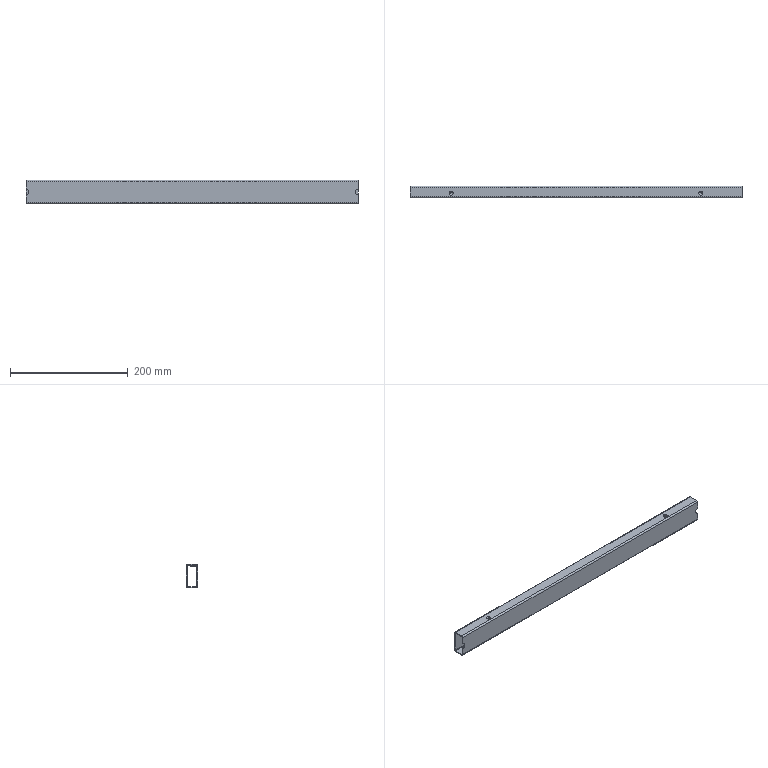Part | STEP file | 7100504 | 1 solid | 29 faces | box 565 x 20 x 40 mm | volume 94145 mm3 | cylinder 14 | plane 12 | torus 3 | commonest cylinder face diameters 2 x4 5 x4 4 x2 10 x2 7 x1 9 x1